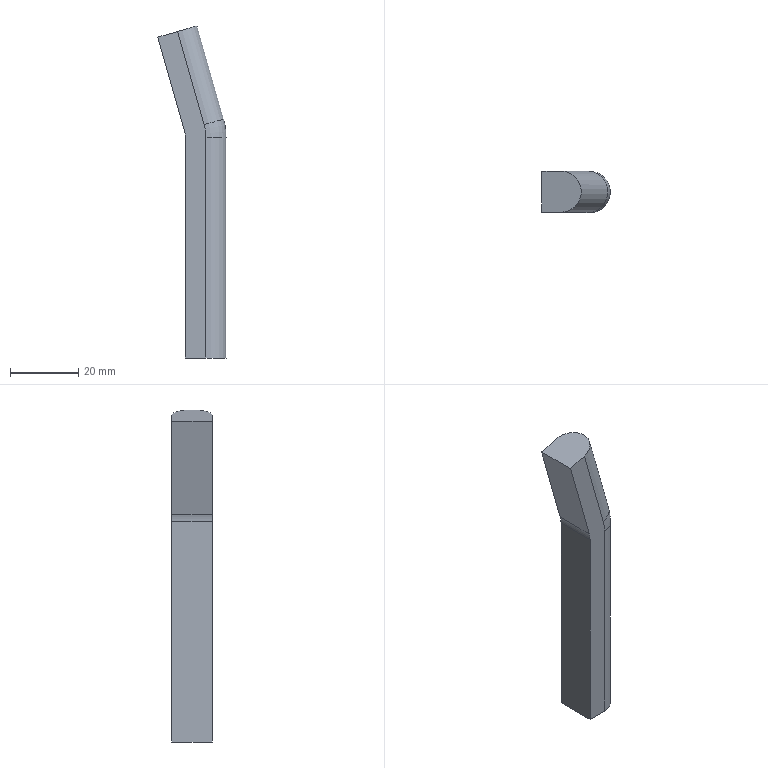Part | NX | features solid 2 | 1 solid | 10 faces | box 20.071 x 12 x 97.272 mm | volume 12419 mm3 | plane 6 | cylinder 3 | torus 1 | commonest cylinder face diameters 12 x2 16 x1
STEP:
#1=CARTESIAN_POINT('',(-887.,-238.5,14.523));
#2=VERTEX_POINT('',#1);
#3=CARTESIAN_POINT('',(-887.,-226.5,14.523));
#4=VERTEX_POINT('',#3);
#5=CARTESIAN_POINT('',(-887.,-202.5,14.523));
#6=DIRECTION('',(0.,1.,0.));
#7=VECTOR('',#6,1000.);
#8=LINE('',#5,#7);
#9=EDGE_CURVE('',#2,#4,#8,.T.);
#10=ORIENTED_EDGE('',*,*,#9,.T.);
#11=CARTESIAN_POINT('',(-887.,-226.5,-50.));
#12=VERTEX_POINT('',#11);
#13=CARTESIAN_POINT('',(-887.,-226.5,39.523));
#14=DIRECTION('',(0.,0.,1.));
#15=VECTOR('',#14,1000.);
#16=LINE('',#13,#15);
#17=EDGE_CURVE('',#12,#4,#16,.T.);
#18=ORIENTED_EDGE('',*,*,#17,.F.);
#19=CARTESIAN_POINT('',(-887.,-238.5,-50.));
#20=VERTEX_POINT('',#19);
#21=CARTESIAN_POINT('',(-887.,-124.5,-50.));
#22=DIRECTION('',(0.,-1.,0.));
#23=VECTOR('',#22,1000.);
#24=LINE('',#21,#23);
#25=EDGE_CURVE('',#12,#20,#24,.T.);
#26=ORIENTED_EDGE('',*,*,#25,.T.);
#27=CARTESIAN_POINT('',(-887.,-238.5,49.523));
#28=DIRECTION('',(0.,0.,-1.));
#29=VECTOR('',#28,1000.);
#30=LINE('',#27,#29);
#31=EDGE_CURVE('',#2,#20,#30,.T.);
#32=ORIENTED_EDGE('',*,*,#31,.F.);
#33=EDGE_LOOP('',(#10,#18,#26,#32));
#34=FACE_BOUND('',#33,.T.);
#35=CARTESIAN_POINT('',(-887.,-202.5,49.523));
#36=DIRECTION('',(1.,0.,0.));
#37=DIRECTION('',(0.,-1.,0.));
#38=AXIS2_PLACEMENT_3D('',#35,#36,#37);
#39=PLANE('',#38);
#40=ADVANCED_FACE('',(#34),#39,.F.);
#41=CARTESIAN_POINT('',(-881.,-226.5,14.523));
#42=VERTEX_POINT('',#41);
#43=CARTESIAN_POINT('',(-881.,-238.5,14.523));
#44=VERTEX_POINT('',#43);
#45=CARTESIAN_POINT('',(-881.,-232.5,14.523));
#46=DIRECTION('',(0.,0.,-1.));
#47=DIRECTION('',(1.,0.,0.));
#48=AXIS2_PLACEMENT_3D('',#45,#46,#47);
#49=CIRCLE('',#48,6.);
#50=EDGE_CURVE('',#42,#44,#49,.T.);
#51=ORIENTED_EDGE('',*,*,#50,.T.);
#52=CARTESIAN_POINT('',(-881.,-238.5,-50.));
#53=VERTEX_POINT('',#52);
#54=CARTESIAN_POINT('',(-881.,-238.5,29.523));
#55=DIRECTION('',(0.,0.,-1.));
#56=VECTOR('',#55,1000.);
#57=LINE('',#54,#56);
#58=EDGE_CURVE('',#44,#53,#57,.T.);
#59=ORIENTED_EDGE('',*,*,#58,.T.);
#60=CARTESIAN_POINT('',(-881.,-226.5,-50.));
#61=VERTEX_POINT('',#60);
#62=CARTESIAN_POINT('',(-881.,-232.5,-50.));
#63=DIRECTION('',(0.,0.,-1.));
#64=DIRECTION('',(0.,-1.,0.));
#65=AXIS2_PLACEMENT_3D('',#62,#63,#64);
#66=CIRCLE('',#65,6.);
#67=EDGE_CURVE('',#61,#53,#66,.T.);
#68=ORIENTED_EDGE('',*,*,#67,.F.);
#69=CARTESIAN_POINT('',(-881.,-226.5,29.523));
#70=DIRECTION('',(0.,0.,-1.));
#71=VECTOR('',#70,1000.);
#72=LINE('',#69,#71);
#73=EDGE_CURVE('',#42,#61,#72,.T.);
#74=ORIENTED_EDGE('',*,*,#73,.F.);
#75=EDGE_LOOP('',(#51,#59,#68,#74));
#76=FACE_BOUND('',#75,.T.);
#77=CARTESIAN_POINT('',(-881.,-232.5,29.523));
#78=DIRECTION('',(0.,0.,-1.));
#79=DIRECTION('',(-1.,0.,0.));
#80=AXIS2_PLACEMENT_3D('',#77,#78,#79);
#81=CYLINDRICAL_SURFACE('',#80,6.);
#82=ADVANCED_FACE('',(#76),#81,.T.);
#83=ORIENTED_EDGE('',*,*,#50,.F.);
#84=CARTESIAN_POINT('',(-881.535,-226.5,18.357));
#85=VERTEX_POINT('',#84);
#86=CARTESIAN_POINT('',(-895.,-226.5,14.523));
#87=DIRECTION('',(0.,-1.,0.));
#88=DIRECTION('',(0.,0.,-1.));
#89=AXIS2_PLACEMENT_3D('',#86,#87,#88);
#90=CIRCLE('',#89,14.);
#91=EDGE_CURVE('',#42,#85,#90,.T.);
#92=ORIENTED_EDGE('',*,*,#91,.T.);
#93=CARTESIAN_POINT('',(-881.535,-238.5,18.357));
#94=VERTEX_POINT('',#93);
#95=CARTESIAN_POINT('',(-881.535,-232.5,18.357));
#96=DIRECTION('',(0.2738,0.,-0.9618));
#97=DIRECTION('',(0.9618,0.,0.2738));
#98=AXIS2_PLACEMENT_3D('',#95,#96,#97);
#99=CIRCLE('',#98,6.);
#100=EDGE_CURVE('',#85,#94,#99,.T.);
#101=ORIENTED_EDGE('',*,*,#100,.T.);
#102=CARTESIAN_POINT('',(-895.,-238.5,14.523));
#103=DIRECTION('',(0.,-1.,0.));
#104=DIRECTION('',(0.,0.,-1.));
#105=AXIS2_PLACEMENT_3D('',#102,#103,#104);
#106=CIRCLE('',#105,14.);
#107=EDGE_CURVE('',#44,#94,#106,.T.);
#108=ORIENTED_EDGE('',*,*,#107,.F.);
#109=EDGE_LOOP('',(#83,#92,#101,#108));
#110=FACE_BOUND('',#109,.T.);
#111=CARTESIAN_POINT('',(-895.,-232.5,14.523));
#112=DIRECTION('',(0.,1.,0.));
#113=DIRECTION('',(0.,0.,-1.));
#114=AXIS2_PLACEMENT_3D('',#111,#112,#113);
#115=TOROIDAL_SURFACE('',#114,14.,6.);
#116=ADVANCED_FACE('',(#110),#115,.T.);
#117=CARTESIAN_POINT('',(-979.,-226.5,-50.));
#118=DIRECTION('',(-1.,0.,0.));
#119=VECTOR('',#118,1000.);
#120=LINE('',#117,#119);
#121=EDGE_CURVE('',#61,#12,#120,.T.);
#122=ORIENTED_EDGE('',*,*,#121,.T.);
#123=ORIENTED_EDGE('',*,*,#17,.T.);
#124=CARTESIAN_POINT('',(-887.306,-226.5,16.714));
#125=VERTEX_POINT('',#124);
#126=CARTESIAN_POINT('',(-895.,-226.5,14.523));
#127=DIRECTION('',(0.,-1.,0.));
#128=DIRECTION('',(0.,0.,-1.));
#129=AXIS2_PLACEMENT_3D('',#126,#127,#128);
#130=CIRCLE('',#129,8.);
#131=EDGE_CURVE('',#4,#125,#130,.T.);
#132=ORIENTED_EDGE('',*,*,#131,.T.);
#133=CARTESIAN_POINT('',(-895.071,-226.5,43.986));
#134=VERTEX_POINT('',#133);
#135=CARTESIAN_POINT('',(-887.306,-226.5,16.714));
#136=DIRECTION('',(-0.2738,0.,0.9618));
#137=VECTOR('',#136,1000.);
#138=LINE('',#135,#137);
#139=EDGE_CURVE('',#125,#134,#138,.T.);
#140=ORIENTED_EDGE('',*,*,#139,.T.);
#141=CARTESIAN_POINT('',(-889.3,-226.5,45.629));
#142=VERTEX_POINT('',#141);
#143=CARTESIAN_POINT('',(-896.81,-226.5,43.491));
#144=DIRECTION('',(-0.9618,0.,-0.2738));
#145=VECTOR('',#144,1000.);
#146=LINE('',#143,#145);
#147=EDGE_CURVE('',#142,#134,#146,.T.);
#148=ORIENTED_EDGE('',*,*,#147,.F.);
#149=CARTESIAN_POINT('',(-881.535,-226.5,18.357));
#150=DIRECTION('',(-0.2738,0.,0.9618));
#151=VECTOR('',#150,1000.);
#152=LINE('',#149,#151);
#153=EDGE_CURVE('',#85,#142,#152,.T.);
#154=ORIENTED_EDGE('',*,*,#153,.F.);
#155=ORIENTED_EDGE('',*,*,#91,.F.);
#156=ORIENTED_EDGE('',*,*,#73,.T.);
#157=EDGE_LOOP('',(#122,#123,#132,#140,#148,#154,#155,#156));
#158=FACE_BOUND('',#157,.T.);
#159=CARTESIAN_POINT('',(-979.,-226.5,39.523));
#160=DIRECTION('',(0.,1.,0.));
#161=DIRECTION('',(1.,0.,0.));
#162=AXIS2_PLACEMENT_3D('',#159,#160,#161);
#163=PLANE('',#162);
#164=ADVANCED_FACE('',(#158),#163,.T.);
#165=CARTESIAN_POINT('',(-889.3,-238.5,45.629));
#166=VERTEX_POINT('',#165);
#167=CARTESIAN_POINT('',(-881.535,-238.5,18.357));
#168=DIRECTION('',(-0.2738,0.,0.9618));
#169=VECTOR('',#168,1000.);
#170=LINE('',#167,#169);
#171=EDGE_CURVE('',#94,#166,#170,.T.);
#172=ORIENTED_EDGE('',*,*,#171,.T.);
#173=CARTESIAN_POINT('',(-895.071,-238.5,43.986));
#174=VERTEX_POINT('',#173);
#175=CARTESIAN_POINT('',(-896.81,-238.5,43.491));
#176=DIRECTION('',(-0.9618,0.,-0.2738));
#177=VECTOR('',#176,1000.);
#178=LINE('',#175,#177);
#179=EDGE_CURVE('',#166,#174,#178,.T.);
#180=ORIENTED_EDGE('',*,*,#179,.T.);
#181=CARTESIAN_POINT('',(-887.306,-238.5,16.714));
#182=VERTEX_POINT('',#181);
#183=CARTESIAN_POINT('',(-887.306,-238.5,16.714));
#184=DIRECTION('',(-0.2738,0.,0.9618));
#185=VECTOR('',#184,1000.);
#186=LINE('',#183,#185);
#187=EDGE_CURVE('',#182,#174,#186,.T.);
#188=ORIENTED_EDGE('',*,*,#187,.F.);
#189=CARTESIAN_POINT('',(-895.,-238.5,14.523));
#190=DIRECTION('',(0.,-1.,0.));
#191=DIRECTION('',(0.,0.,-1.));
#192=AXIS2_PLACEMENT_3D('',#189,#190,#191);
#193=CIRCLE('',#192,8.);
#194=EDGE_CURVE('',#2,#182,#193,.T.);
#195=ORIENTED_EDGE('',*,*,#194,.F.);
#196=ORIENTED_EDGE('',*,*,#31,.T.);
#197=CARTESIAN_POINT('',(-979.,-238.5,-50.));
#198=DIRECTION('',(-1.,0.,0.));
#199=VECTOR('',#198,1000.);
#200=LINE('',#197,#199);
#201=EDGE_CURVE('',#53,#20,#200,.T.);
#202=ORIENTED_EDGE('',*,*,#201,.F.);
#203=ORIENTED_EDGE('',*,*,#58,.F.);
#204=ORIENTED_EDGE('',*,*,#107,.T.);
#205=EDGE_LOOP('',(#172,#180,#188,#195,#196,#202,#203,#204));
#206=FACE_BOUND('',#205,.T.);
#207=CARTESIAN_POINT('',(-979.,-238.5,39.523));
#208=DIRECTION('',(0.,1.,0.));
#209=DIRECTION('',(1.,0.,0.));
#210=AXIS2_PLACEMENT_3D('',#207,#208,#209);
#211=PLANE('',#210);
#212=ADVANCED_FACE('',(#206),#211,.F.);
#213=CARTESIAN_POINT('',(-889.3,-232.5,45.629));
#214=DIRECTION('',(-0.2738,0.,0.9618));
#215=DIRECTION('',(0.9618,0.,0.2738));
#216=AXIS2_PLACEMENT_3D('',#213,#214,#215);
#217=CIRCLE('',#216,6.);
#218=EDGE_CURVE('',#142,#166,#217,.F.);
#219=ORIENTED_EDGE('',*,*,#218,.F.);
#220=ORIENTED_EDGE('',*,*,#147,.T.);
#221=CARTESIAN_POINT('',(-895.071,-202.5,43.986));
#222=DIRECTION('',(0.,1.,0.));
#223=VECTOR('',#222,1000.);
#224=LINE('',#221,#223);
#225=EDGE_CURVE('',#174,#134,#224,.T.);
#226=ORIENTED_EDGE('',*,*,#225,.F.);
#227=ORIENTED_EDGE('',*,*,#179,.F.);
#228=EDGE_LOOP('',(#219,#220,#226,#227));
#229=FACE_BOUND('',#228,.T.);
#230=CARTESIAN_POINT('',(-896.81,-172.75,43.491));
#231=DIRECTION('',(-0.2738,0.,0.9618));
#232=DIRECTION('',(0.9618,0.,0.2738));
#233=AXIS2_PLACEMENT_3D('',#230,#231,#232);
#234=PLANE('',#233);
#235=ADVANCED_FACE('',(#229),#234,.T.);
#236=ORIENTED_EDGE('',*,*,#218,.T.);
#237=ORIENTED_EDGE('',*,*,#171,.F.);
#238=ORIENTED_EDGE('',*,*,#100,.F.);
#239=ORIENTED_EDGE('',*,*,#153,.T.);
#240=EDGE_LOOP('',(#236,#237,#238,#239));
#241=FACE_BOUND('',#240,.T.);
#242=CARTESIAN_POINT('',(-881.535,-232.5,18.357));
#243=DIRECTION('',(-0.2738,0.,0.9618));
#244=DIRECTION('',(0.9618,0.,0.2738));
#245=AXIS2_PLACEMENT_3D('',#242,#243,#244);
#246=CYLINDRICAL_SURFACE('',#245,6.);
#247=ADVANCED_FACE('',(#241),#246,.T.);
#248=ORIENTED_EDGE('',*,*,#25,.F.);
#249=ORIENTED_EDGE('',*,*,#121,.F.);
#250=ORIENTED_EDGE('',*,*,#67,.T.);
#251=ORIENTED_EDGE('',*,*,#201,.T.);
#252=EDGE_LOOP('',(#248,#249,#250,#251));
#253=FACE_BOUND('',#252,.T.);
#254=CARTESIAN_POINT('',(-932.,-124.5,-50.));
#255=DIRECTION('',(0.,0.,1.));
#256=DIRECTION('',(1.,0.,0.));
#257=AXIS2_PLACEMENT_3D('',#254,#255,#256);
#258=PLANE('',#257);
#259=ADVANCED_FACE('',(#253),#258,.F.);
#260=CARTESIAN_POINT('',(-887.306,-202.5,16.714));
#261=DIRECTION('',(0.,1.,0.));
#262=VECTOR('',#261,1000.);
#263=LINE('',#260,#262);
#264=EDGE_CURVE('',#182,#125,#263,.T.);
#265=ORIENTED_EDGE('',*,*,#264,.F.);
#266=ORIENTED_EDGE('',*,*,#187,.T.);
#267=ORIENTED_EDGE('',*,*,#225,.T.);
#268=ORIENTED_EDGE('',*,*,#139,.F.);
#269=EDGE_LOOP('',(#265,#266,#267,#268));
#270=FACE_BOUND('',#269,.T.);
#271=CARTESIAN_POINT('',(-887.306,-202.5,16.714));
#272=DIRECTION('',(-0.9618,0.,-0.2738));
#273=DIRECTION('',(-0.2738,0.,0.9618));
#274=AXIS2_PLACEMENT_3D('',#271,#272,#273);
#275=PLANE('',#274);
#276=ADVANCED_FACE('',(#270),#275,.T.);
#277=ORIENTED_EDGE('',*,*,#9,.F.);
#278=ORIENTED_EDGE('',*,*,#194,.T.);
#279=ORIENTED_EDGE('',*,*,#264,.T.);
#280=ORIENTED_EDGE('',*,*,#131,.F.);
#281=EDGE_LOOP('',(#277,#278,#279,#280));
#282=FACE_BOUND('',#281,.T.);
#283=CARTESIAN_POINT('',(-895.,-187.5,14.523));
#284=DIRECTION('',(0.,1.,0.));
#285=DIRECTION('',(0.,0.,-1.));
#286=AXIS2_PLACEMENT_3D('',#283,#284,#285);
#287=CYLINDRICAL_SURFACE('',#286,8.);
#288=ADVANCED_FACE('',(#282),#287,.F.);
#289=CLOSED_SHELL('',(#40,#82,#116,#164,#212,#235,#247,#259,#276,#288));
#290=MANIFOLD_SOLID_BREP('',#289);
#291=(LENGTH_UNIT()NAMED_UNIT(*)SI_UNIT(.MILLI.,.METRE.));
#292=UNCERTAINTY_MEASURE_WITH_UNIT(LENGTH_MEASURE(0.00001),#291,'','');
#293=(NAMED_UNIT(*)PLANE_ANGLE_UNIT()SI_UNIT($,.RADIAN.));
#294=(NAMED_UNIT(*)SI_UNIT($,.STERADIAN.)SOLID_ANGLE_UNIT());
#295=(GEOMETRIC_REPRESENTATION_CONTEXT(3)GLOBAL_UNCERTAINTY_ASSIGNED_CONTEXT((#292))GLOBAL_UNIT_ASSIGNED_CONTEXT((#291,#293,#294))REPRESENTATION_CONTEXT('',''));
#296=ADVANCED_BREP_SHAPE_REPRESENTATION('',(#290),#295);